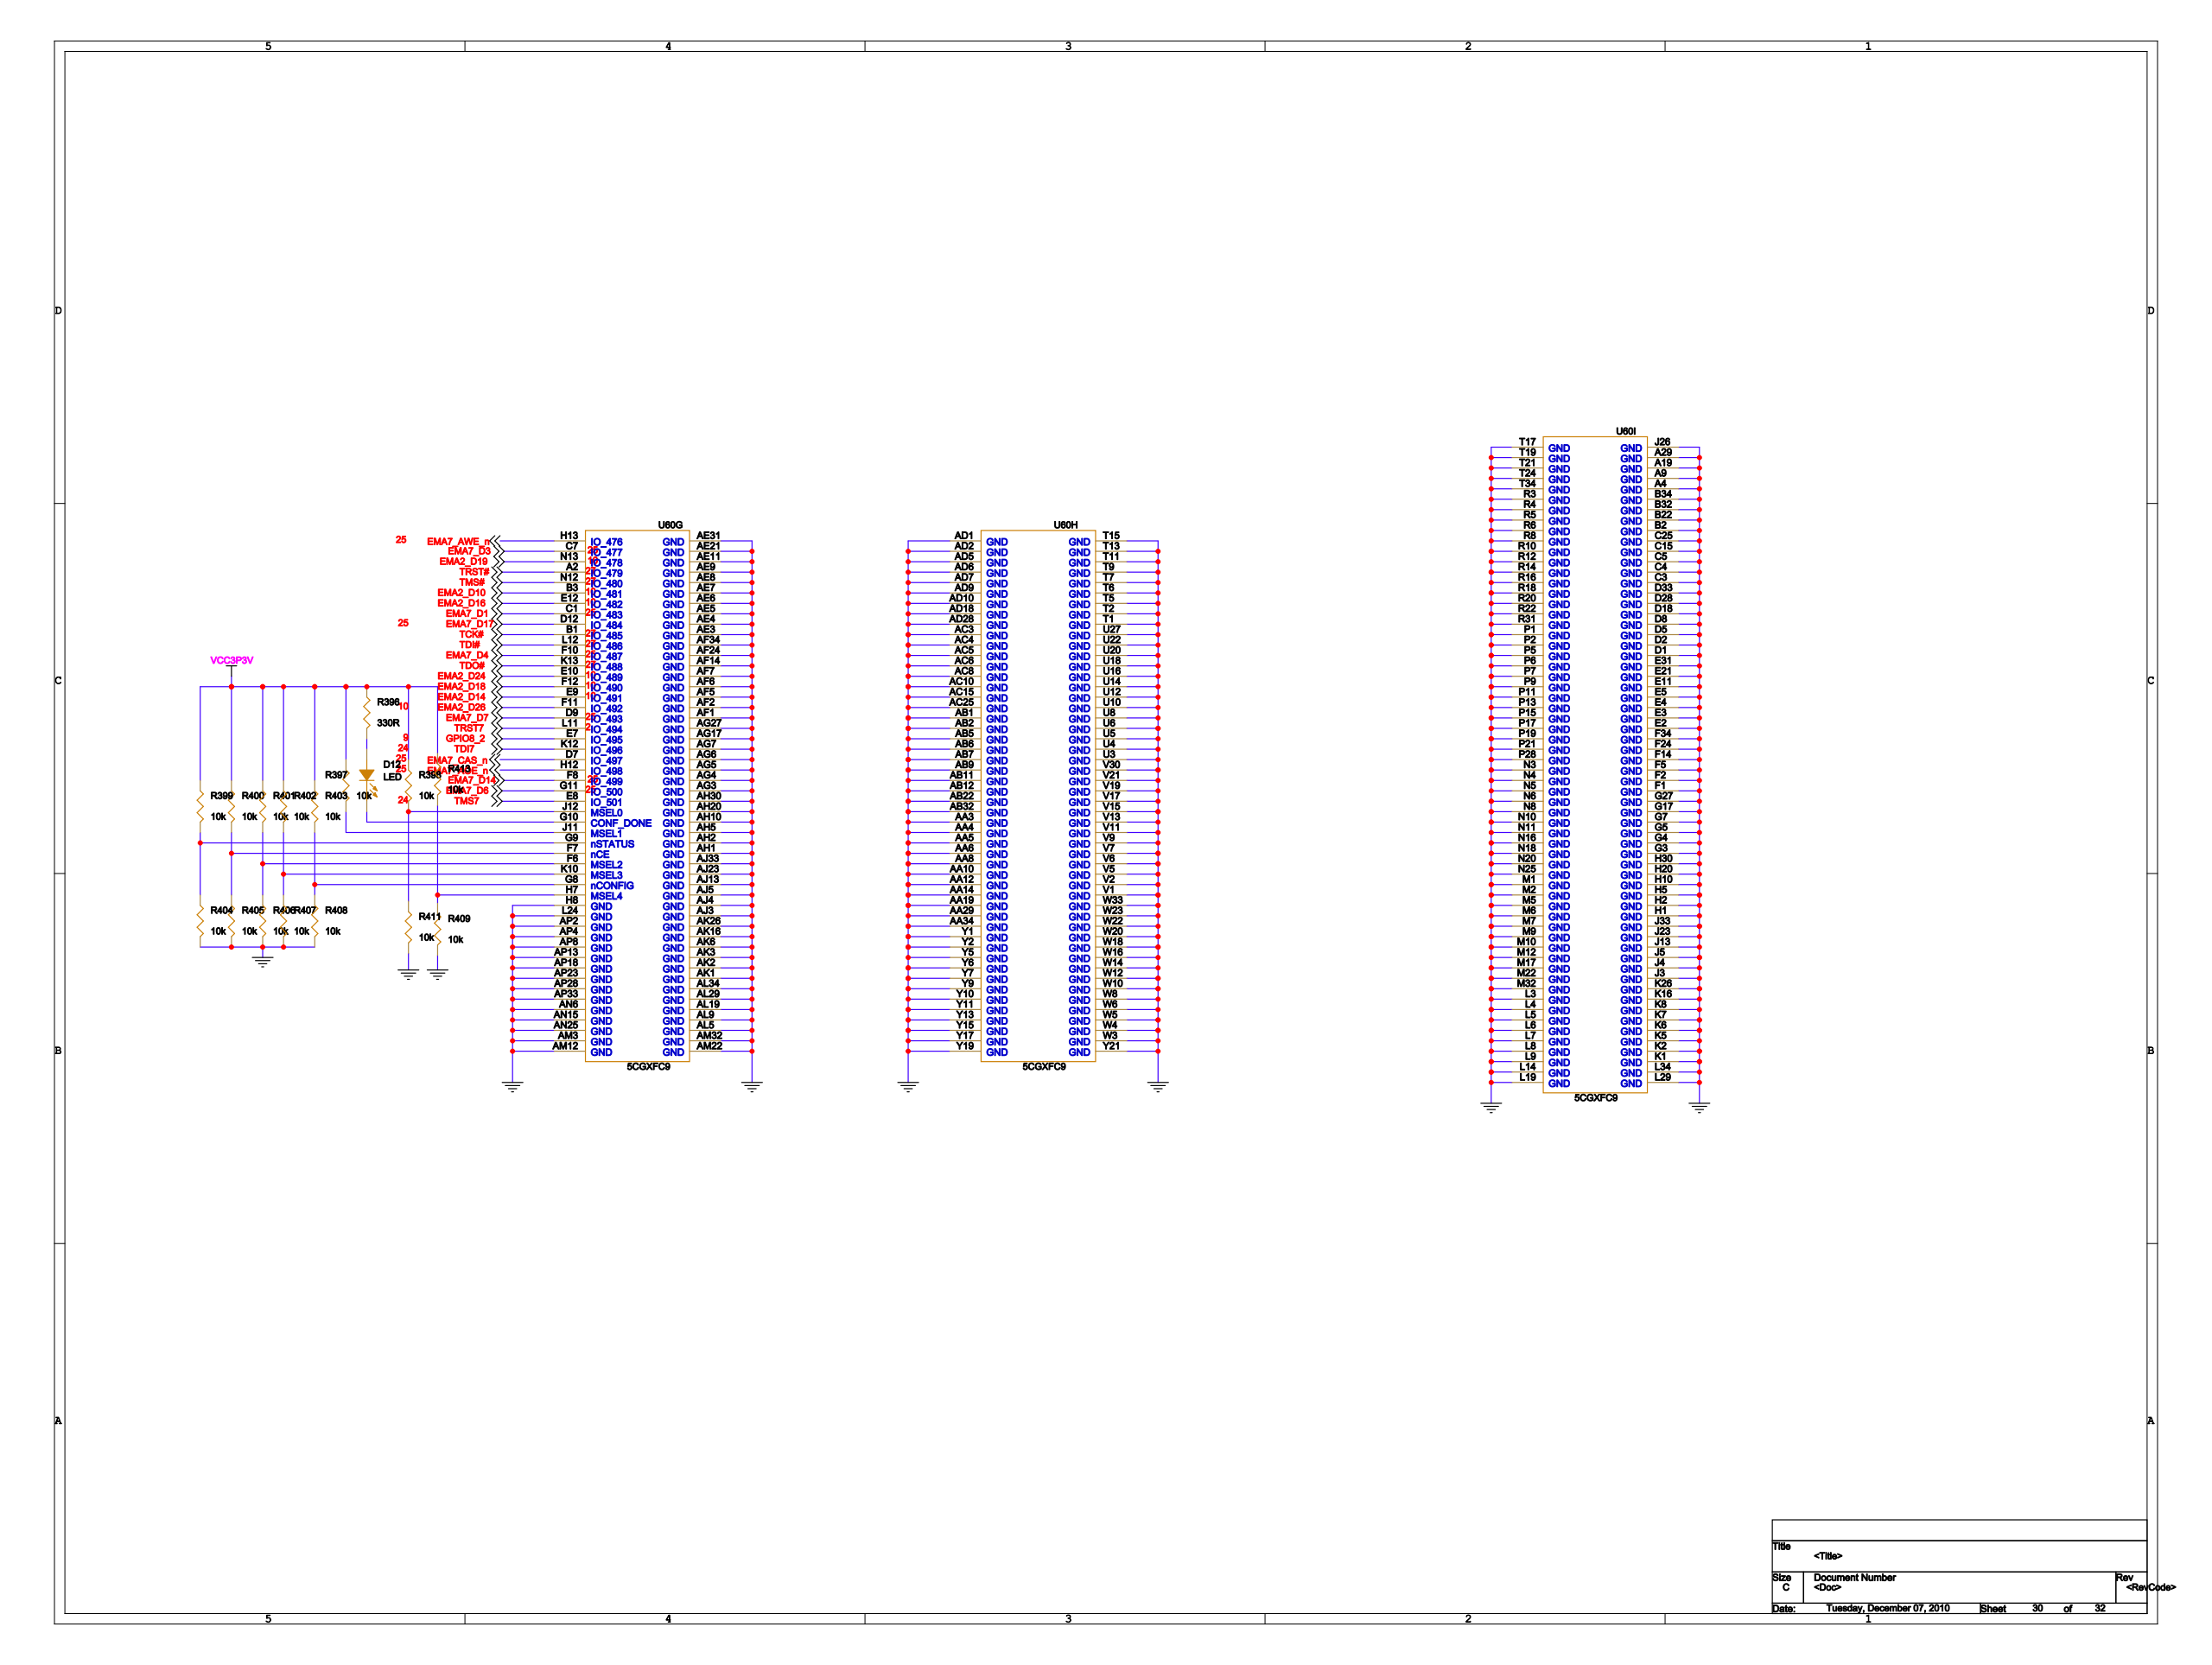Circuit board | Cadence Allegro | 1001 parts | 1318 nets | one sheet of the schematic
Parts on this sheet (reference | value | footprint):
D12 | LED | LED0805
R396 | 330R | 0603
R397 | 10K | 0603
R398 | 10K | 0603
R399 | 10K | 0603
R400 | 10K | 0603
R401 | 10K | 0603
R402 | 10K | 0603
R403 | 10K | 0603
R404 | 10K | 0603
R405 | 10K | 0603
R406 | 10K | 0603
R407 | 10K | 0603
R408 | 10K | 0603
R409 | 10K | 0603
R411 | 10K | 0603
R413 | 10K | 0603
U4 | MAX3243 | TSSOP-28
U6 | MT48LC16M16 | TSOP54
U8 | DP83848C | DP83848C_48LQFP
U10 | SoC_HTC_01 | L529_XIN
U14 | MT48LC16M16 | TSOP54
U16 | SoC_HTC_01 | L529_XIN
U20 | MT48LC16M16 | TSOP54
U22 | SoC_HTC_01 | L529_XIN
U27 | MT48LC16M16 | TSOP54
U60 | 5CGXFC9 | FBGA1152
Nets of these parts (net: part-pin ...):
N17056676: D12-2 U60-G10
GND: R404-2 R405-2 R406-2 R407-2 R408-2 R409-2 R411-2 U4-25 U10-AA3 U10-AA12 U10-D2 U10-D5 U10-E12 U10-E21 U10-G4 U10-G5 U10-G10 U10-H10 U10-H13 U10-J13 U10-K7 U10-L5 U10-L6 U10-L9 U10-M6 U10-M7 U10-N5 U10-N18 U10-P9 U10-R4 U10-R16 U10-R18 U10-T5 U10-T9 U10-T17 U10-U5 U10-U6 U10-U8 U10-V9 U10-V11 U10-W4 U10-W10 U10-W16 U10-W18 U10-Y15 U10-Y19 U16-AA3 U16-AA12 U16-D2 U16-D5 U16-E12 U16-E21 U16-G4 U16-G5 U16-G10 U16-H10 U16-H13 U16-J13 U16-K7 U16-L5 U16-L6 U16-L9 U16-M6 U16-M7 U16-N5 U16-N18 U16-P9 U16-R4 U16-R16 U16-R18 U16-T5 U16-T9 U16-T17 U16-U5 U16-U6 U16-U8 U16-V9 U16-V11 U16-W4 U16-W10 U16-W16 U16-W18 U16-Y15 U16-Y19 U22-AA3 U22-AA12 U22-D2 U22-D5 U22-E12 U22-E21 U22-G4 U22-G5 U22-G10 U22-H10 U22-H13 U22-J13 U22-K7 U22-L5 U22-L6 U22-L9 U22-M6 U22-M7 U22-N5 U22-N18 U22-P9 U22-R4 U22-R16 U22-R18 U22-T5 U22-T9 U22-T17 U22-U5 U22-U6 U22-U8 U22-V9 U22-V11 U22-W4 U22-W10 U22-W16 U22-W18 U22-Y15 U22-Y19 U60-A4 U60-A9 U60-A19 U60-A29 U60-AA3 U60-AA4 U60-AA5 U60-AA6 U60-AA8 U60-AA10 U60-AA12 U60-AA14 U60-AA19 U60-AA29 U60-AA34 U60-AB1 U60-AB2 U60-AB5 U60-AB6 U60-AB7 U60-AB9 U60-AB11 U60-AB12 U60-AB22 U60-AB32 U60-AC3 U60-AC4 U60-AC5 U60-AC6 U60-AC8 U60-AC10 U60-AC15 U60-AC25 U60-AD1 U60-AD2 U60-AD5 U60-AD6 U60-AD7 U60-AD9 U60-AD10 U60-AD18 U60-AD28 U60-AE3 U60-AE4 U60-AE5 U60-AE6 U60-AE7 U60-AE8 U60-AE9 U60-AE11 U60-AE21 U60-AE31 U60-AF1 U60-AF2 U60-AF5 U60-AF6 U60-AF7 U60-AF14 U60-AF24 U60-AF34 U60-AG3 U60-AG4 U60-AG5 U60-AG6 U60-AG7 U60-AG17 U60-AG27 U60-AH1 U60-AH2 U60-AH5 U60-AH10 U60-AH20 U60-AH30 U60-AJ3 U60-AJ4 U60-AJ5 U60-AJ13 U60-AJ23 U60-AJ33 U60-AK1 U60-AK2 U60-AK3 U60-AK6 U60-AK16 U60-AK26 U60-AL5 U60-AL9 U60-AL19 U60-AL29 U60-AL34 U60-AM3 U60-AM12 U60-AM22 U60-AM32 U60-AN6 U60-AN15 U60-AN25 U60-AP2 U60-AP4 U60-AP8 U60-AP13 U60-AP18 U60-AP23 U60-AP28 U60-AP33 U60-B2 U60-B22 U60-B32 U60-B34 U60-C3 U60-C4 U60-C5 U60-C15 U60-C25 U60-D1 U60-D2 U60-D5 U60-D8 U60-D18 U60-D28 U60-D33 U60-E2 U60-E3 U60-E4 U60-E5 U60-E11 U60-E21 U60-E31 U60-F1 U60-F2 U60-F5 U60-F14 U60-F24 U60-F34 U60-G3 U60-G4 U60-G5 U60-G7 U60-G17 U60-G27 U60-H1 U60-H2 U60-H5 U60-H8 U60-H10 U60-H20 U60-H30 U60-J3 U60-J4 U60-J5 U60-J13 U60-J23 U60-J26 U60-J33 U60-K1 U60-K2 U60-K5 U60-K6 U60-K7 U60-K8 U60-K16 U60-K26 U60-L3 U60-L4 U60-L5 U60-L6 U60-L7 U60-L8 U60-L9 U60-L14 U60-L19 U60-L24 U60-L29 U60-L34 U60-M1 U60-M2 U60-M5 U60-M6 U60-M7 U60-M9 U60-M10 U60-M12 U60-M17 U60-M22 U60-M32 U60-N3 U60-N4 U60-N5 U60-N6 U60-N8 U60-N10 U60-N11 U60-N16 U60-N18 U60-N20 U60-N25 U60-P1 U60-P2 U60-P5 U60-P6 U60-P7 U60-P9 U60-P11 U60-P13 U60-P15 U60-P17 U60-P19 U60-P21 U60-P28 U60-R3 U60-R4 U60-R5 U60-R6 U60-R8 U60-R10 U60-R12 U60-R14 U60-R16 U60-R18 U60-R20 U60-R22 U60-R31 U60-T1 U60-T2 U60-T5 U60-T6 U60-T7 U60-T9 U60-T11 U60-T13 U60-T15 U60-T17 U60-T19 U60-T21 U60-T24 U60-T34 U60-U3 U60-U4 U60-U5 U60-U6 U60-U8 U60-U10 U60-U12 U60-U14 U60-U16 U60-U18 U60-U20 U60-U22 U60-U27 U60-V1 U60-V2 U60-V5 U60-V6 U60-V7 U60-V9 U60-V11 U60-V13 U60-V15 U60-V17 U60-V19 U60-V21 U60-V30 U60-W3 U60-W4 U60-W5 U60-W6 U60-W8 U60-W10 U60-W12 U60-W14 U60-W16 U60-W18 U60-W20 U60-W22 U60-W23 U60-W33 U60-Y1 U60-Y2 U60-Y5 U60-Y6 U60-Y7 U60-Y9 U60-Y10 U60-Y11 U60-Y13 U60-Y15 U60-Y17 U60-Y19 U60-Y21
TRST#: U60-A2
TCK#: U60-B1
EMA2_D10: U60-B3
EMA7_D1: U60-C1
EMA7_D3: U60-C7
EMA7_D17: U60-D12
EMA7_D7: U60-D9
EMA2_D24: U60-E10
EMA2_D16: U60-E12
GPIO8_2: U60-E7
TMS7: U60-E8
EMA2_D14: U16-U14 U60-E9
EMA7_D4: U60-F10
EMA2_D26: U16-T15 U60-F11
EMA2_D18: U16-R14 U60-F12
EMA7_D14: U60-F8
EMA7_D6: U60-G11
TDI7: U60-K12
TDO#: U60-K13
TRST7: U60-L11
TDI#: U60-L12
TMS#: U60-N12
EMA2_D19: U60-N13
N17056673: R398-2 R411-1 U60-J12
N17056681: R397-2 U60-J11
N17064431: R401-2 R406-1 U60-F6
N17064420: R402-2 R407-1 U60-K10
N17072769: R409-1 R413-2 U60-H7
N17064442: R400-2 R405-1 U60-F7
N17064409: R403-2 R408-1 U60-G8
N17064462: R399-2 R404-1 U60-G9
VCC3P3V: R396-1 R397-1 R398-1 R399-1 R400-1 R401-1 R402-1 R403-1 R413-1 U4-22 U6-9 U6-27 U8-22 U8-32 U10-AA14 U10-AB2 U10-AB11 U10-B3 U10-B22 U10-C1 U10-E11 U10-F7 U10-G17 U10-H7 U10-J4 U10-K8 U10-N4 U10-P15 U10-R5 U10-U10 U10-W3 U10-Y7 U10-Y13 U10-Y17 U14-9 U14-27 U16-AA14 U16-AB2 U16-AB11 U16-B3 U16-B22 U16-C1 U16-E11 U16-F7 U16-G17 U16-H7 U16-J4 U16-K8 U16-N4 U16-P15 U16-R5 U16-U10 U16-W3 U16-Y7 U16-Y13 U16-Y17 U20-9 U20-27 U22-AA14 U22-AB2 U22-AB11 U22-B3 U22-B22 U22-C1 U22-E11 U22-F7 U22-G17 U22-H7 U22-J4 U22-K8 U22-N4 U22-P15 U22-R5 U22-U10 U22-W3 U22-Y7 U22-Y13 U22-Y17 U27-9 U27-27
N17654965: D12-1 R396-2